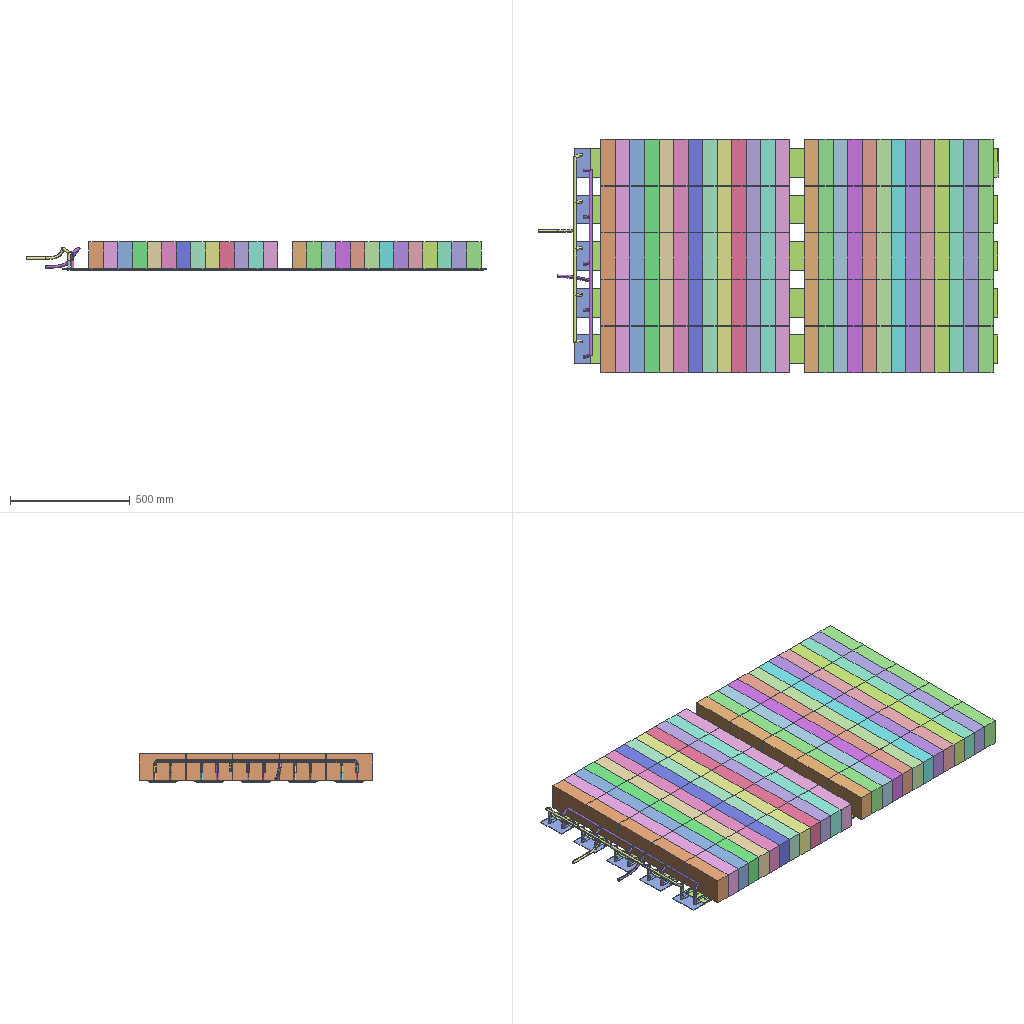Assembly | SolidWorks | 33 different items | 157 placed | box 1923 x 975 x 120 mm
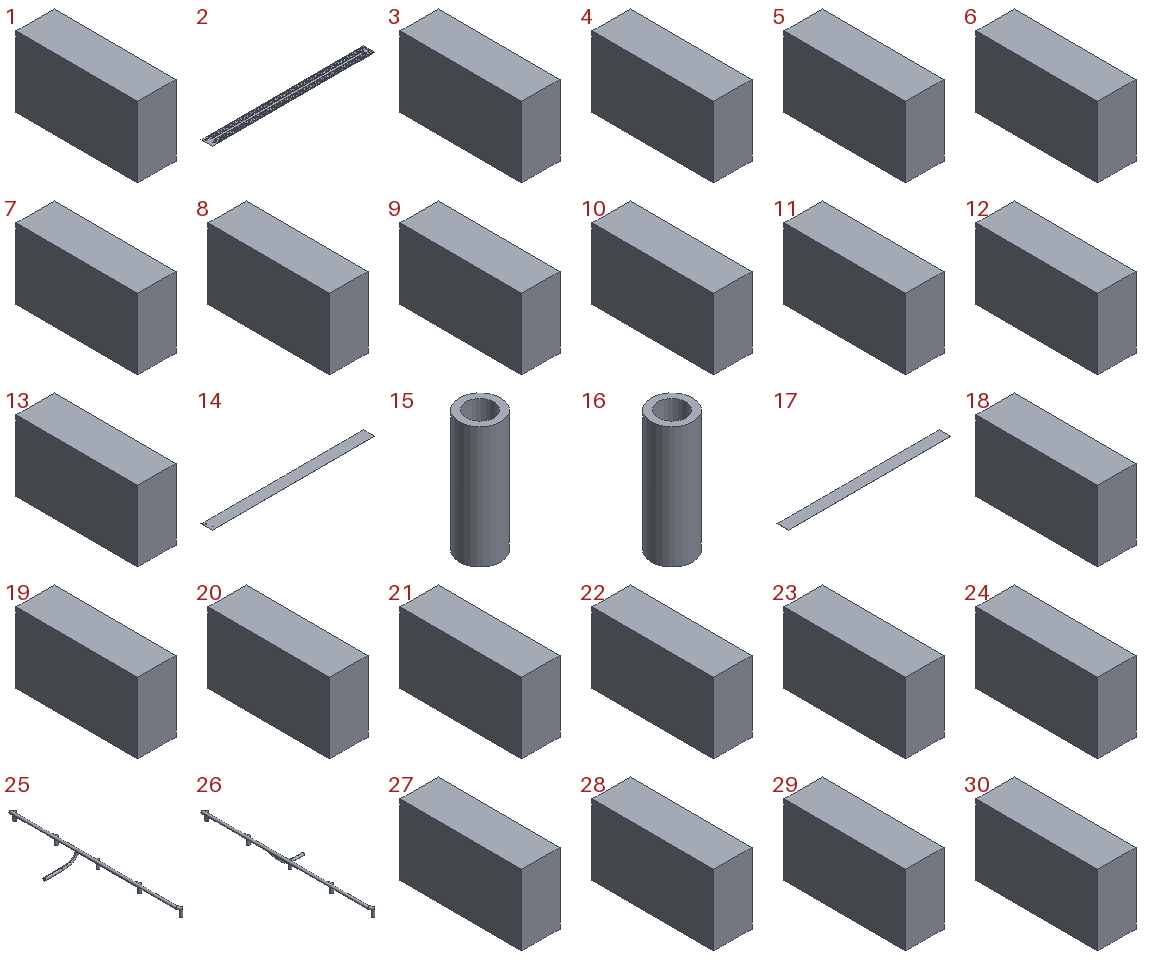Parts list (item | quantity | size | volume | features):
1 | x5 | 60.7 x 194.65 x 112.8 mm | 1332761 mm3 | features BaseBody 1
2 | x5 | 1768 x 120 x 5 mm | 286159 mm3 | features ICE 7, LPattern 2, BaseBody 1
3 | x5 | 60.7 x 194.65 x 112.8 mm | 1332761 mm3 | features BaseBody 1
4 | x5 | 60.7 x 194.65 x 112.8 mm | 1332761 mm3 | features BaseBody 1
5 | x5 | 60.7 x 194.65 x 112.8 mm | 1332761 mm3 | features BaseBody 1
6 | x5 | 60.7 x 194.65 x 112.8 mm | 1332761 mm3 | features BaseBody 1
7 | x5 | 60.7 x 194.65 x 112.8 mm | 1332761 mm3 | features BaseBody 1
8 | x5 | 60.7 x 194.65 x 112.8 mm | 1332761 mm3 | features BaseBody 1
9 | x5 | 60.7 x 194.65 x 112.8 mm | 1332761 mm3 | features BaseBody 1
10 | x5 | 60.7 x 194.65 x 112.8 mm | 1332761 mm3 | features BaseBody 1
11 | x5 | 60.7 x 194.65 x 112.8 mm | 1332761 mm3 | features BaseBody 1
12 | x5 | 60.7 x 194.65 x 112.8 mm | 1332761 mm3 | features BaseBody 1
13 | x5 | 60.7 x 194.65 x 112.8 mm | 1332761 mm3 | features BaseBody 1
14 | x5 | 1768 x 120 x 1 mm | 211934 mm3 | features BaseBody 1
15 | x5 | 12 x 12 x 35 mm | 2199 mm3 | features BaseBody 1
16 | x5 | 12 x 12 x 35 mm | 2199 mm3 | features BaseBody 1
17 | x5 | 1703 x 120 x 1 mm | 204360 mm3 | features BaseBody 1
18 | x5 | 60.7 x 194.65 x 112.8 mm | 1332761 mm3 | features BaseBody 1
19 | x5 | 60.7 x 194.65 x 112.8 mm | 1332761 mm3 | features BaseBody 1
20 | x5 | 60.7 x 194.65 x 112.8 mm | 1332761 mm3 | features BaseBody 1
21 | x5 | 60.7 x 194.65 x 112.8 mm | 1332761 mm3 | features BaseBody 1
22 | x5 | 60.7 x 194.65 x 112.8 mm | 1332761 mm3 | features BaseBody 1
23 | x5 | 60.7 x 194.65 x 112.8 mm | 1332761 mm3 | features BaseBody 1
24 | x5 | 60.7 x 194.65 x 112.8 mm | 1332761 mm3 | features BaseBody 1
25 | x1 | 185.606 x 792 x 56.756 mm | 78943 mm3 | features Sweep 5, 3DProfileFeature 2
26 | x1 | 146.397 x 792 x 87.372 mm | 78940 mm3 | features Sweep 5, 3DProfileFeature 2
27 | x5 | 60.7 x 194.65 x 112.8 mm | 1332761 mm3 | features BaseBody 1
28 | x5 | 60.7 x 194.65 x 112.8 mm | 1332761 mm3 | features BaseBody 1
29 | x5 | 60.7 x 194.65 x 112.8 mm | 1332761 mm3 | features BaseBody 1
30 | x5 | 60.7 x 194.65 x 112.8 mm | 1332761 mm3 | features BaseBody 1
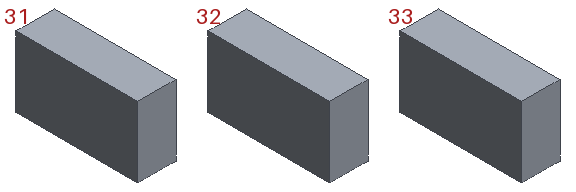31 | x5 | 60.7 x 194.65 x 112.8 mm | 1332761 mm3 | features BaseBody 1
32 | x5 | 60.7 x 194.65 x 112.8 mm | 1332761 mm3 | features BaseBody 1
33 | x5 | 60.7 x 194.65 x 112.8 mm | 1332761 mm3 | features BaseBody 1
Mates (type | each side: item.copy, entity, surface, feature):
Concentric | 16.1 face cylinder Input 1 | 25.1 face cylinder Sweep-Thin Part 1
Concentric | 16.2 face cylinder Input 1 | 25.1 face cylinder Sweep-Thin Part 1
Concentric | 15.1 face cylinder Input 1 | 26.1 face cylinder Sweep-Thin Part 1
Concentric | 15.2 face cylinder Input 1 | 26.1 face cylinder Sweep-Thin Part 4
Coincident | 15.1 face plane Input 1 | 26.1 face plane Sweep-Thin Part 1
Coincident | 16.1 face plane Input 1 | 25.1 face plane Sweep-Thin Part 1